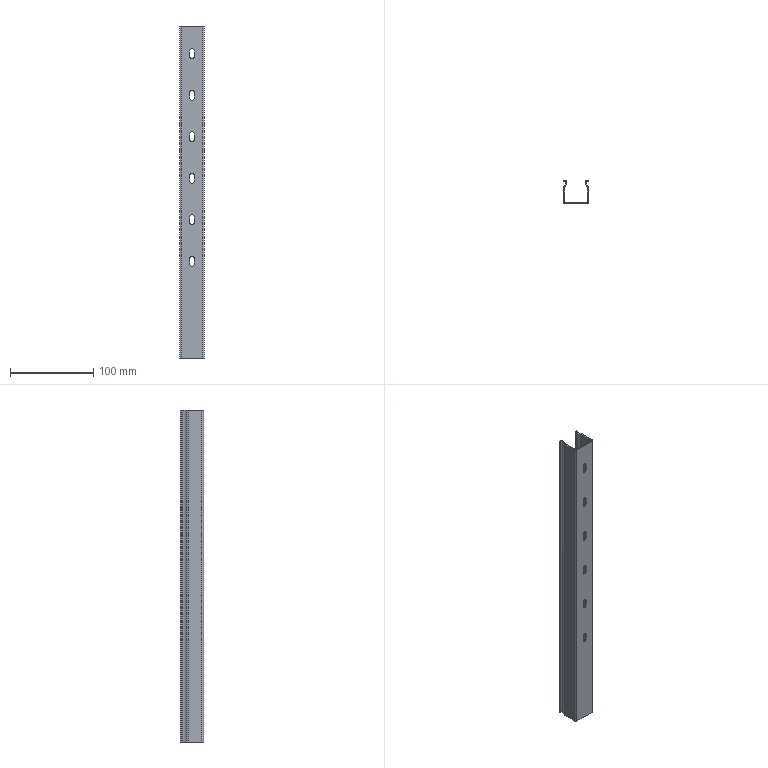Part | SolidWorks | features BaseBody 1 | 1 solid | 62 faces | box 30 x 28 x 400 mm | volume 43012 mm3 | cylinder 36 | plane 26 | commonest cylinder face diameters 5 x18 2 x3 4.5 x3 1.5 x2 3.5 x2 4 x2